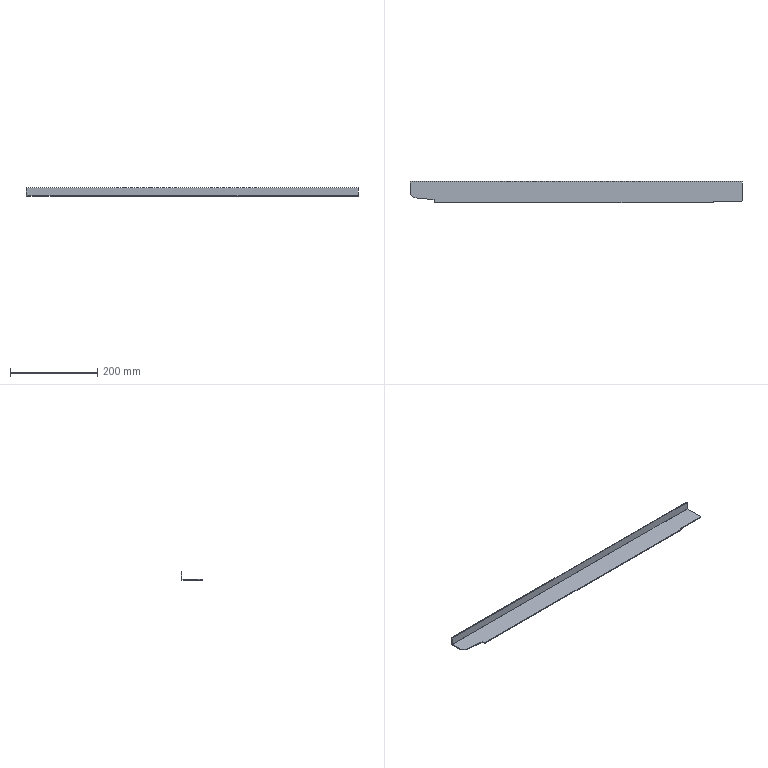Part | SolidWorks | 1 solid | 21 faces | box 759.5 x 50 x 20 mm | volume 100833 mm3 | plane 19 | cylinder 2 | commonest cylinder face diameters 0.2 x1 4.2 x1
STEP:
#1=CARTESIAN_POINT('',(-379.75,22.9,-2.));
#2=VERTEX_POINT('',#1);
#3=CARTESIAN_POINT('',(-379.75,-3.027,-2.));
#4=VERTEX_POINT('',#3);
#5=CARTESIAN_POINT('',(-379.75,-25.,-2.));
#6=DIRECTION('',(0.,-1.,0.));
#7=VECTOR('',#6,1000.);
#8=LINE('',#5,#7);
#9=EDGE_CURVE('',#2,#4,#8,.T.);
#10=ORIENTED_EDGE('',*,*,#9,.T.);
#11=CARTESIAN_POINT('',(-379.75,-3.027,0.));
#12=VERTEX_POINT('',#11);
#13=CARTESIAN_POINT('',(-379.75,-3.027,-2.));
#14=DIRECTION('',(0.,0.,1.));
#15=VECTOR('',#14,1000.);
#16=LINE('',#13,#15);
#17=EDGE_CURVE('',#4,#12,#16,.T.);
#18=ORIENTED_EDGE('',*,*,#17,.T.);
#19=CARTESIAN_POINT('',(-379.75,22.9,0.));
#20=VERTEX_POINT('',#19);
#21=CARTESIAN_POINT('',(-379.75,-25.,0.));
#22=DIRECTION('',(0.,-1.,0.));
#23=VECTOR('',#22,1000.);
#24=LINE('',#21,#23);
#25=EDGE_CURVE('',#20,#12,#24,.T.);
#26=ORIENTED_EDGE('',*,*,#25,.F.);
#27=CARTESIAN_POINT('',(-379.75,22.9,0.));
#28=DIRECTION('',(0.,0.,-1.));
#29=VECTOR('',#28,1000.);
#30=LINE('',#27,#29);
#31=EDGE_CURVE('',#20,#2,#30,.T.);
#32=ORIENTED_EDGE('',*,*,#31,.T.);
#33=EDGE_LOOP('',(#10,#18,#26,#32));
#34=FACE_OUTER_BOUND('',#33,.T.);
#35=CARTESIAN_POINT('',(-379.75,-25.,-2.));
#36=DIRECTION('',(-1.,0.,0.));
#37=DIRECTION('',(0.,0.,1.));
#38=AXIS2_PLACEMENT_3D('',#35,#36,#37);
#39=PLANE('',#38);
#40=ADVANCED_FACE('',(#34),#39,.T.);
#41=CARTESIAN_POINT('',(-323.25,-25.,-2.));
#42=VERTEX_POINT('',#41);
#43=CARTESIAN_POINT('',(-323.25,-17.499,-2.));
#44=VERTEX_POINT('',#43);
#45=CARTESIAN_POINT('',(-323.25,0.,-2.));
#46=DIRECTION('',(0.,1.,0.));
#47=VECTOR('',#46,1000.);
#48=LINE('',#45,#47);
#49=EDGE_CURVE('',#42,#44,#48,.T.);
#50=ORIENTED_EDGE('',*,*,#49,.T.);
#51=CARTESIAN_POINT('',(-327.727,-17.499,-2.));
#52=VERTEX_POINT('',#51);
#53=CARTESIAN_POINT('',(0.,-17.499,-2.));
#54=DIRECTION('',(-1.,0.,0.));
#55=VECTOR('',#54,1000.);
#56=LINE('',#53,#55);
#57=EDGE_CURVE('',#44,#52,#56,.T.);
#58=ORIENTED_EDGE('',*,*,#57,.T.);
#59=CARTESIAN_POINT('',(-370.795,-12.972,-2.));
#60=VERTEX_POINT('',#59);
#61=CARTESIAN_POINT('',(-5.4,-51.377,-2.));
#62=DIRECTION('',(-0.9945,0.1045,0.));
#63=VECTOR('',#62,1000.);
#64=LINE('',#61,#63);
#65=EDGE_CURVE('',#52,#60,#64,.T.);
#66=ORIENTED_EDGE('',*,*,#65,.T.);
#67=CARTESIAN_POINT('',(-211.227,-190.19,-2.));
#68=DIRECTION('',(-0.6691,0.7431,0.));
#69=VECTOR('',#68,1000.);
#70=LINE('',#67,#69);
#71=EDGE_CURVE('',#60,#4,#70,.T.);
#72=ORIENTED_EDGE('',*,*,#71,.T.);
#73=ORIENTED_EDGE('',*,*,#9,.F.);
#74=CARTESIAN_POINT('',(379.75,22.9,-2.));
#75=VERTEX_POINT('',#74);
#76=CARTESIAN_POINT('',(-379.75,22.9,-2.));
#77=DIRECTION('',(1.,0.,0.));
#78=VECTOR('',#77,1000.);
#79=LINE('',#76,#78);
#80=EDGE_CURVE('',#2,#75,#79,.T.);
#81=ORIENTED_EDGE('',*,*,#80,.T.);
#82=CARTESIAN_POINT('',(379.75,-20.,-2.));
#83=VERTEX_POINT('',#82);
#84=CARTESIAN_POINT('',(379.75,-25.,-2.));
#85=DIRECTION('',(0.,1.,0.));
#86=VECTOR('',#85,1000.);
#87=LINE('',#84,#86);
#88=EDGE_CURVE('',#83,#75,#87,.T.);
#89=ORIENTED_EDGE('',*,*,#88,.F.);
#90=CARTESIAN_POINT('',(378.75,-21.,-2.));
#91=VERTEX_POINT('',#90);
#92=CARTESIAN_POINT('',(199.875,-199.875,-2.));
#93=DIRECTION('',(-0.7071,-0.7071,0.));
#94=VECTOR('',#93,1000.);
#95=LINE('',#92,#94);
#96=EDGE_CURVE('',#83,#91,#95,.T.);
#97=ORIENTED_EDGE('',*,*,#96,.T.);
#98=CARTESIAN_POINT('',(313.75,-21.,-2.));
#99=VERTEX_POINT('',#98);
#100=CARTESIAN_POINT('',(0.,-21.,-2.));
#101=DIRECTION('',(-1.,0.,0.));
#102=VECTOR('',#101,1000.);
#103=LINE('',#100,#102);
#104=EDGE_CURVE('',#91,#99,#103,.T.);
#105=ORIENTED_EDGE('',*,*,#104,.T.);
#106=CARTESIAN_POINT('',(313.75,-25.,-2.));
#107=VERTEX_POINT('',#106);
#108=CARTESIAN_POINT('',(313.75,0.,-2.));
#109=DIRECTION('',(0.,-1.,0.));
#110=VECTOR('',#109,1000.);
#111=LINE('',#108,#110);
#112=EDGE_CURVE('',#99,#107,#111,.T.);
#113=ORIENTED_EDGE('',*,*,#112,.T.);
#114=CARTESIAN_POINT('',(379.75,-25.,-2.));
#115=DIRECTION('',(1.,0.,0.));
#116=VECTOR('',#115,1000.);
#117=LINE('',#114,#116);
#118=EDGE_CURVE('',#42,#107,#117,.T.);
#119=ORIENTED_EDGE('',*,*,#118,.F.);
#120=EDGE_LOOP('',(#50,#58,#66,#72,#73,#81,#89,#97,#105,#113,#119));
#121=FACE_OUTER_BOUND('',#120,.T.);
#122=CARTESIAN_POINT('',(0.,0.,-2.));
#123=DIRECTION('',(0.,0.,1.));
#124=DIRECTION('',(1.,0.,0.));
#125=AXIS2_PLACEMENT_3D('',#122,#123,#124);
#126=PLANE('',#125);
#127=ADVANCED_FACE('',(#121),#126,.F.);
#128=CARTESIAN_POINT('',(-323.25,-17.499,0.));
#129=VERTEX_POINT('',#128);
#130=CARTESIAN_POINT('',(-327.727,-17.499,0.));
#131=VERTEX_POINT('',#130);
#132=CARTESIAN_POINT('',(0.,-17.499,0.));
#133=DIRECTION('',(-1.,0.,0.));
#134=VECTOR('',#133,1000.);
#135=LINE('',#132,#134);
#136=EDGE_CURVE('',#129,#131,#135,.T.);
#137=ORIENTED_EDGE('',*,*,#136,.F.);
#138=CARTESIAN_POINT('',(-323.25,-25.,0.));
#139=VERTEX_POINT('',#138);
#140=CARTESIAN_POINT('',(-323.25,0.,0.));
#141=DIRECTION('',(0.,1.,0.));
#142=VECTOR('',#141,1000.);
#143=LINE('',#140,#142);
#144=EDGE_CURVE('',#139,#129,#143,.T.);
#145=ORIENTED_EDGE('',*,*,#144,.F.);
#146=CARTESIAN_POINT('',(313.75,-25.,0.));
#147=VERTEX_POINT('',#146);
#148=CARTESIAN_POINT('',(379.75,-25.,0.));
#149=DIRECTION('',(1.,0.,0.));
#150=VECTOR('',#149,1000.);
#151=LINE('',#148,#150);
#152=EDGE_CURVE('',#139,#147,#151,.T.);
#153=ORIENTED_EDGE('',*,*,#152,.T.);
#154=CARTESIAN_POINT('',(313.75,-21.,0.));
#155=VERTEX_POINT('',#154);
#156=CARTESIAN_POINT('',(313.75,0.,0.));
#157=DIRECTION('',(0.,-1.,0.));
#158=VECTOR('',#157,1000.);
#159=LINE('',#156,#158);
#160=EDGE_CURVE('',#155,#147,#159,.T.);
#161=ORIENTED_EDGE('',*,*,#160,.F.);
#162=CARTESIAN_POINT('',(378.75,-21.,0.));
#163=VERTEX_POINT('',#162);
#164=CARTESIAN_POINT('',(0.,-21.,0.));
#165=DIRECTION('',(-1.,0.,0.));
#166=VECTOR('',#165,1000.);
#167=LINE('',#164,#166);
#168=EDGE_CURVE('',#163,#155,#167,.T.);
#169=ORIENTED_EDGE('',*,*,#168,.F.);
#170=CARTESIAN_POINT('',(379.75,-20.,0.));
#171=VERTEX_POINT('',#170);
#172=CARTESIAN_POINT('',(199.875,-199.875,0.));
#173=DIRECTION('',(-0.7071,-0.7071,0.));
#174=VECTOR('',#173,1000.);
#175=LINE('',#172,#174);
#176=EDGE_CURVE('',#171,#163,#175,.T.);
#177=ORIENTED_EDGE('',*,*,#176,.F.);
#178=CARTESIAN_POINT('',(379.75,22.9,0.));
#179=VERTEX_POINT('',#178);
#180=CARTESIAN_POINT('',(379.75,-25.,0.));
#181=DIRECTION('',(0.,1.,0.));
#182=VECTOR('',#181,1000.);
#183=LINE('',#180,#182);
#184=EDGE_CURVE('',#171,#179,#183,.T.);
#185=ORIENTED_EDGE('',*,*,#184,.T.);
#186=CARTESIAN_POINT('',(-379.75,22.9,0.));
#187=DIRECTION('',(1.,0.,0.));
#188=VECTOR('',#187,1000.);
#189=LINE('',#186,#188);
#190=EDGE_CURVE('',#20,#179,#189,.T.);
#191=ORIENTED_EDGE('',*,*,#190,.F.);
#192=ORIENTED_EDGE('',*,*,#25,.T.);
#193=CARTESIAN_POINT('',(-370.795,-12.972,0.));
#194=VERTEX_POINT('',#193);
#195=CARTESIAN_POINT('',(-211.227,-190.19,0.));
#196=DIRECTION('',(-0.6691,0.7431,0.));
#197=VECTOR('',#196,1000.);
#198=LINE('',#195,#197);
#199=EDGE_CURVE('',#194,#12,#198,.T.);
#200=ORIENTED_EDGE('',*,*,#199,.F.);
#201=CARTESIAN_POINT('',(-5.4,-51.377,0.));
#202=DIRECTION('',(-0.9945,0.1045,0.));
#203=VECTOR('',#202,1000.);
#204=LINE('',#201,#203);
#205=EDGE_CURVE('',#131,#194,#204,.T.);
#206=ORIENTED_EDGE('',*,*,#205,.F.);
#207=EDGE_LOOP('',(#137,#145,#153,#161,#169,#177,#185,#191,#192,#200,#206));
#208=FACE_OUTER_BOUND('',#207,.T.);
#209=CARTESIAN_POINT('',(0.,0.,0.));
#210=DIRECTION('',(0.,0.,1.));
#211=DIRECTION('',(1.,0.,0.));
#212=AXIS2_PLACEMENT_3D('',#209,#210,#211);
#213=PLANE('',#212);
#214=ADVANCED_FACE('',(#208),#213,.T.);
#215=ORIENTED_EDGE('',*,*,#184,.F.);
#216=CARTESIAN_POINT('',(379.75,-20.,-2.));
#217=DIRECTION('',(0.,0.,1.));
#218=VECTOR('',#217,1000.);
#219=LINE('',#216,#218);
#220=EDGE_CURVE('',#83,#171,#219,.T.);
#221=ORIENTED_EDGE('',*,*,#220,.F.);
#222=ORIENTED_EDGE('',*,*,#88,.T.);
#223=CARTESIAN_POINT('',(379.75,22.9,0.));
#224=DIRECTION('',(0.,0.,-1.));
#225=VECTOR('',#224,1000.);
#226=LINE('',#223,#225);
#227=EDGE_CURVE('',#179,#75,#226,.T.);
#228=ORIENTED_EDGE('',*,*,#227,.F.);
#229=EDGE_LOOP('',(#215,#221,#222,#228));
#230=FACE_OUTER_BOUND('',#229,.T.);
#231=CARTESIAN_POINT('',(379.75,-25.,-2.));
#232=DIRECTION('',(1.,0.,0.));
#233=DIRECTION('',(0.,0.,-1.));
#234=AXIS2_PLACEMENT_3D('',#231,#232,#233);
#235=PLANE('',#234);
#236=ADVANCED_FACE('',(#230),#235,.T.);
#237=ORIENTED_EDGE('',*,*,#152,.F.);
#238=CARTESIAN_POINT('',(-323.25,-25.,-2.));
#239=DIRECTION('',(0.,0.,1.));
#240=VECTOR('',#239,1000.);
#241=LINE('',#238,#240);
#242=EDGE_CURVE('',#42,#139,#241,.T.);
#243=ORIENTED_EDGE('',*,*,#242,.F.);
#244=ORIENTED_EDGE('',*,*,#118,.T.);
#245=CARTESIAN_POINT('',(313.75,-25.,-2.));
#246=DIRECTION('',(0.,0.,1.));
#247=VECTOR('',#246,1000.);
#248=LINE('',#245,#247);
#249=EDGE_CURVE('',#107,#147,#248,.T.);
#250=ORIENTED_EDGE('',*,*,#249,.T.);
#251=EDGE_LOOP('',(#237,#243,#244,#250));
#252=FACE_OUTER_BOUND('',#251,.T.);
#253=CARTESIAN_POINT('',(379.75,-25.,-2.));
#254=DIRECTION('',(0.,-1.,0.));
#255=DIRECTION('',(1.,0.,0.));
#256=AXIS2_PLACEMENT_3D('',#253,#254,#255);
#257=PLANE('',#256);
#258=ADVANCED_FACE('',(#252),#257,.T.);
#259=CARTESIAN_POINT('',(379.75,23.,0.1));
#260=VERTEX_POINT('',#259);
#261=CARTESIAN_POINT('',(379.75,25.,0.1));
#262=VERTEX_POINT('',#261);
#263=CARTESIAN_POINT('',(379.75,25.,0.1));
#264=DIRECTION('',(0.,1.,0.));
#265=VECTOR('',#264,1000.);
#266=LINE('',#263,#265);
#267=EDGE_CURVE('',#260,#262,#266,.T.);
#268=ORIENTED_EDGE('',*,*,#267,.F.);
#269=CARTESIAN_POINT('',(379.75,22.9,0.1));
#270=DIRECTION('',(1.,0.,0.));
#271=DIRECTION('',(0.,0.,1.));
#272=AXIS2_PLACEMENT_3D('',#269,#270,#271);
#273=CIRCLE('',#272,0.1);
#274=EDGE_CURVE('',#179,#260,#273,.T.);
#275=ORIENTED_EDGE('',*,*,#274,.F.);
#276=ORIENTED_EDGE('',*,*,#227,.T.);
#277=CARTESIAN_POINT('',(379.75,22.9,0.1));
#278=DIRECTION('',(1.,0.,0.));
#279=DIRECTION('',(0.,0.,1.));
#280=AXIS2_PLACEMENT_3D('',#277,#278,#279);
#281=CIRCLE('',#280,2.1);
#282=EDGE_CURVE('',#75,#262,#281,.T.);
#283=ORIENTED_EDGE('',*,*,#282,.T.);
#284=EDGE_LOOP('',(#268,#275,#276,#283));
#285=FACE_OUTER_BOUND('',#284,.T.);
#286=CARTESIAN_POINT('',(379.75,22.9,0.1));
#287=DIRECTION('',(1.,0.,0.));
#288=DIRECTION('',(0.,0.,-1.));
#289=AXIS2_PLACEMENT_3D('',#286,#287,#288);
#290=PLANE('',#289);
#291=ADVANCED_FACE('',(#285),#290,.T.);
#292=CARTESIAN_POINT('',(-379.75,23.,0.1));
#293=VERTEX_POINT('',#292);
#294=CARTESIAN_POINT('',(-379.75,22.9,0.1));
#295=DIRECTION('',(-1.,0.,0.));
#296=DIRECTION('',(0.,0.,1.));
#297=AXIS2_PLACEMENT_3D('',#294,#295,#296);
#298=CIRCLE('',#297,0.1);
#299=EDGE_CURVE('',#293,#20,#298,.T.);
#300=ORIENTED_EDGE('',*,*,#299,.F.);
#301=CARTESIAN_POINT('',(-379.75,25.,0.1));
#302=VERTEX_POINT('',#301);
#303=CARTESIAN_POINT('',(-379.75,23.,0.1));
#304=DIRECTION('',(0.,1.,0.));
#305=VECTOR('',#304,1000.);
#306=LINE('',#303,#305);
#307=EDGE_CURVE('',#293,#302,#306,.T.);
#308=ORIENTED_EDGE('',*,*,#307,.T.);
#309=CARTESIAN_POINT('',(-379.75,22.9,0.1));
#310=DIRECTION('',(-1.,0.,0.));
#311=DIRECTION('',(0.,0.,1.));
#312=AXIS2_PLACEMENT_3D('',#309,#310,#311);
#313=CIRCLE('',#312,2.1);
#314=EDGE_CURVE('',#302,#2,#313,.T.);
#315=ORIENTED_EDGE('',*,*,#314,.T.);
#316=ORIENTED_EDGE('',*,*,#31,.F.);
#317=EDGE_LOOP('',(#300,#308,#315,#316));
#318=FACE_OUTER_BOUND('',#317,.T.);
#319=CARTESIAN_POINT('',(-379.75,22.9,0.1));
#320=DIRECTION('',(1.,0.,0.));
#321=DIRECTION('',(0.,0.,-1.));
#322=AXIS2_PLACEMENT_3D('',#319,#320,#321);
#323=PLANE('',#322);
#324=ADVANCED_FACE('',(#318),#323,.F.);
#325=ORIENTED_EDGE('',*,*,#80,.F.);
#326=ORIENTED_EDGE('',*,*,#314,.F.);
#327=CARTESIAN_POINT('',(379.75,25.,0.1));
#328=DIRECTION('',(1.,0.,0.));
#329=VECTOR('',#328,1000.);
#330=LINE('',#327,#329);
#331=EDGE_CURVE('',#302,#262,#330,.T.);
#332=ORIENTED_EDGE('',*,*,#331,.T.);
#333=ORIENTED_EDGE('',*,*,#282,.F.);
#334=EDGE_LOOP('',(#325,#326,#332,#333));
#335=FACE_OUTER_BOUND('',#334,.T.);
#336=CARTESIAN_POINT('',(-379.75,22.9,0.1));
#337=DIRECTION('',(-1.,0.,0.));
#338=DIRECTION('',(0.,1.,0.));
#339=AXIS2_PLACEMENT_3D('',#336,#337,#338);
#340=CYLINDRICAL_SURFACE('',#339,2.1);
#341=ADVANCED_FACE('',(#335),#340,.T.);
#342=ORIENTED_EDGE('',*,*,#190,.T.);
#343=ORIENTED_EDGE('',*,*,#274,.T.);
#344=CARTESIAN_POINT('',(379.75,23.,0.1));
#345=DIRECTION('',(-1.,0.,0.));
#346=VECTOR('',#345,1000.);
#347=LINE('',#344,#346);
#348=EDGE_CURVE('',#260,#293,#347,.T.);
#349=ORIENTED_EDGE('',*,*,#348,.T.);
#350=ORIENTED_EDGE('',*,*,#299,.T.);
#351=EDGE_LOOP('',(#342,#343,#349,#350));
#352=FACE_OUTER_BOUND('',#351,.T.);
#353=CARTESIAN_POINT('',(-379.75,22.9,0.1));
#354=DIRECTION('',(-1.,0.,0.));
#355=DIRECTION('',(0.,1.,0.));
#356=AXIS2_PLACEMENT_3D('',#353,#354,#355);
#357=CYLINDRICAL_SURFACE('',#356,0.1);
#358=ADVANCED_FACE('',(#352),#357,.F.);
#359=ORIENTED_EDGE('',*,*,#267,.T.);
#360=CARTESIAN_POINT('',(379.75,25.,18.));
#361=VERTEX_POINT('',#360);
#362=CARTESIAN_POINT('',(379.75,25.,0.));
#363=DIRECTION('',(0.,0.,-1.));
#364=VECTOR('',#363,1000.);
#365=LINE('',#362,#364);
#366=EDGE_CURVE('',#361,#262,#365,.T.);
#367=ORIENTED_EDGE('',*,*,#366,.F.);
#368=CARTESIAN_POINT('',(379.75,23.,18.));
#369=VERTEX_POINT('',#368);
#370=CARTESIAN_POINT('',(379.75,25.,18.));
#371=DIRECTION('',(0.,-1.,0.));
#372=VECTOR('',#371,1000.);
#373=LINE('',#370,#372);
#374=EDGE_CURVE('',#361,#369,#373,.T.);
#375=ORIENTED_EDGE('',*,*,#374,.T.);
#376=CARTESIAN_POINT('',(379.75,23.,0.));
#377=DIRECTION('',(0.,0.,-1.));
#378=VECTOR('',#377,1000.);
#379=LINE('',#376,#378);
#380=EDGE_CURVE('',#369,#260,#379,.T.);
#381=ORIENTED_EDGE('',*,*,#380,.T.);
#382=EDGE_LOOP('',(#359,#367,#375,#381));
#383=FACE_OUTER_BOUND('',#382,.T.);
#384=CARTESIAN_POINT('',(379.75,25.,0.));
#385=DIRECTION('',(-1.,0.,0.));
#386=DIRECTION('',(0.,-1.,0.));
#387=AXIS2_PLACEMENT_3D('',#384,#385,#386);
#388=PLANE('',#387);
#389=ADVANCED_FACE('',(#383),#388,.F.);
#390=ORIENTED_EDGE('',*,*,#307,.F.);
#391=CARTESIAN_POINT('',(-379.75,23.,18.));
#392=VERTEX_POINT('',#391);
#393=CARTESIAN_POINT('',(-379.75,23.,18.));
#394=DIRECTION('',(0.,0.,1.));
#395=VECTOR('',#394,1000.);
#396=LINE('',#393,#395);
#397=EDGE_CURVE('',#293,#392,#396,.T.);
#398=ORIENTED_EDGE('',*,*,#397,.T.);
#399=CARTESIAN_POINT('',(-379.75,25.,18.));
#400=VERTEX_POINT('',#399);
#401=CARTESIAN_POINT('',(-379.75,25.,18.));
#402=DIRECTION('',(0.,-1.,0.));
#403=VECTOR('',#402,1000.);
#404=LINE('',#401,#403);
#405=EDGE_CURVE('',#400,#392,#404,.T.);
#406=ORIENTED_EDGE('',*,*,#405,.F.);
#407=CARTESIAN_POINT('',(-379.75,25.,0.));
#408=DIRECTION('',(0.,0.,1.));
#409=VECTOR('',#408,1000.);
#410=LINE('',#407,#409);
#411=EDGE_CURVE('',#302,#400,#410,.T.);
#412=ORIENTED_EDGE('',*,*,#411,.F.);
#413=EDGE_LOOP('',(#390,#398,#406,#412));
#414=FACE_OUTER_BOUND('',#413,.T.);
#415=CARTESIAN_POINT('',(-379.75,25.,18.));
#416=DIRECTION('',(1.,0.,0.));
#417=DIRECTION('',(0.,1.,0.));
#418=AXIS2_PLACEMENT_3D('',#415,#416,#417);
#419=PLANE('',#418);
#420=ADVANCED_FACE('',(#414),#419,.F.);
#421=ORIENTED_EDGE('',*,*,#331,.F.);
#422=ORIENTED_EDGE('',*,*,#411,.T.);
#423=CARTESIAN_POINT('',(0.,25.,18.));
#424=DIRECTION('',(1.,0.,0.));
#425=VECTOR('',#424,1000.);
#426=LINE('',#423,#425);
#427=EDGE_CURVE('',#400,#361,#426,.T.);
#428=ORIENTED_EDGE('',*,*,#427,.T.);
#429=ORIENTED_EDGE('',*,*,#366,.T.);
#430=EDGE_LOOP('',(#421,#422,#428,#429));
#431=FACE_OUTER_BOUND('',#430,.T.);
#432=CARTESIAN_POINT('',(0.,25.,0.));
#433=DIRECTION('',(0.,-1.,0.));
#434=DIRECTION('',(0.,0.,-1.));
#435=AXIS2_PLACEMENT_3D('',#432,#433,#434);
#436=PLANE('',#435);
#437=ADVANCED_FACE('',(#431),#436,.F.);
#438=ORIENTED_EDGE('',*,*,#397,.F.);
#439=ORIENTED_EDGE('',*,*,#348,.F.);
#440=ORIENTED_EDGE('',*,*,#380,.F.);
#441=CARTESIAN_POINT('',(379.75,23.,18.));
#442=DIRECTION('',(1.,0.,0.));
#443=VECTOR('',#442,1000.);
#444=LINE('',#441,#443);
#445=EDGE_CURVE('',#392,#369,#444,.T.);
#446=ORIENTED_EDGE('',*,*,#445,.F.);
#447=EDGE_LOOP('',(#438,#439,#440,#446));
#448=FACE_OUTER_BOUND('',#447,.T.);
#449=CARTESIAN_POINT('',(0.,23.,0.));
#450=DIRECTION('',(0.,-1.,0.));
#451=DIRECTION('',(0.,0.,-1.));
#452=AXIS2_PLACEMENT_3D('',#449,#450,#451);
#453=PLANE('',#452);
#454=ADVANCED_FACE('',(#448),#453,.T.);
#455=ORIENTED_EDGE('',*,*,#445,.T.);
#456=ORIENTED_EDGE('',*,*,#374,.F.);
#457=ORIENTED_EDGE('',*,*,#427,.F.);
#458=ORIENTED_EDGE('',*,*,#405,.T.);
#459=EDGE_LOOP('',(#455,#456,#457,#458));
#460=FACE_OUTER_BOUND('',#459,.T.);
#461=CARTESIAN_POINT('',(379.75,25.,18.));
#462=DIRECTION('',(0.,0.,-1.));
#463=DIRECTION('',(0.,1.,0.));
#464=AXIS2_PLACEMENT_3D('',#461,#462,#463);
#465=PLANE('',#464);
#466=ADVANCED_FACE('',(#460),#465,.F.);
#467=ORIENTED_EDGE('',*,*,#249,.F.);
#468=ORIENTED_EDGE('',*,*,#112,.F.);
#469=CARTESIAN_POINT('',(313.75,-21.,-2.));
#470=DIRECTION('',(0.,0.,1.));
#471=VECTOR('',#470,1000.);
#472=LINE('',#469,#471);
#473=EDGE_CURVE('',#99,#155,#472,.T.);
#474=ORIENTED_EDGE('',*,*,#473,.T.);
#475=ORIENTED_EDGE('',*,*,#160,.T.);
#476=EDGE_LOOP('',(#467,#468,#474,#475));
#477=FACE_OUTER_BOUND('',#476,.T.);
#478=CARTESIAN_POINT('',(313.75,0.,-2.));
#479=DIRECTION('',(-1.,0.,0.));
#480=DIRECTION('',(0.,-1.,0.));
#481=AXIS2_PLACEMENT_3D('',#478,#479,#480);
#482=PLANE('',#481);
#483=ADVANCED_FACE('',(#477),#482,.F.);
#484=ORIENTED_EDGE('',*,*,#473,.F.);
#485=ORIENTED_EDGE('',*,*,#104,.F.);
#486=CARTESIAN_POINT('',(378.75,-21.,-2.));
#487=DIRECTION('',(0.,0.,1.));
#488=VECTOR('',#487,1000.);
#489=LINE('',#486,#488);
#490=EDGE_CURVE('',#91,#163,#489,.T.);
#491=ORIENTED_EDGE('',*,*,#490,.T.);
#492=ORIENTED_EDGE('',*,*,#168,.T.);
#493=EDGE_LOOP('',(#484,#485,#491,#492));
#494=FACE_OUTER_BOUND('',#493,.T.);
#495=CARTESIAN_POINT('',(0.,-21.,-2.));
#496=DIRECTION('',(0.,1.,0.));
#497=DIRECTION('',(-1.,0.,0.));
#498=AXIS2_PLACEMENT_3D('',#495,#496,#497);
#499=PLANE('',#498);
#500=ADVANCED_FACE('',(#494),#499,.F.);
#501=ORIENTED_EDGE('',*,*,#490,.F.);
#502=ORIENTED_EDGE('',*,*,#96,.F.);
#503=ORIENTED_EDGE('',*,*,#220,.T.);
#504=ORIENTED_EDGE('',*,*,#176,.T.);
#505=EDGE_LOOP('',(#501,#502,#503,#504));
#506=FACE_OUTER_BOUND('',#505,.T.);
#507=CARTESIAN_POINT('',(199.875,-199.875,-2.));
#508=DIRECTION('',(-0.7071,0.7071,0.));
#509=DIRECTION('',(-0.7071,-0.7071,0.));
#510=AXIS2_PLACEMENT_3D('',#507,#508,#509);
#511=PLANE('',#510);
#512=ADVANCED_FACE('',(#506),#511,.F.);
#513=CARTESIAN_POINT('',(-327.727,-17.499,-2.));
#514=DIRECTION('',(0.,0.,1.));
#515=VECTOR('',#514,1000.);
#516=LINE('',#513,#515);
#517=EDGE_CURVE('',#52,#131,#516,.T.);
#518=ORIENTED_EDGE('',*,*,#517,.F.);
#519=ORIENTED_EDGE('',*,*,#57,.F.);
#520=CARTESIAN_POINT('',(-323.25,-17.499,-2.));
#521=DIRECTION('',(0.,0.,1.));
#522=VECTOR('',#521,1000.);
#523=LINE('',#520,#522);
#524=EDGE_CURVE('',#44,#129,#523,.T.);
#525=ORIENTED_EDGE('',*,*,#524,.T.);
#526=ORIENTED_EDGE('',*,*,#136,.T.);
#527=EDGE_LOOP('',(#518,#519,#525,#526));
#528=FACE_OUTER_BOUND('',#527,.T.);
#529=CARTESIAN_POINT('',(0.,-17.499,-2.));
#530=DIRECTION('',(0.,1.,0.));
#531=DIRECTION('',(-1.,0.,0.));
#532=AXIS2_PLACEMENT_3D('',#529,#530,#531);
#533=PLANE('',#532);
#534=ADVANCED_FACE('',(#528),#533,.F.);
#535=ORIENTED_EDGE('',*,*,#524,.F.);
#536=ORIENTED_EDGE('',*,*,#49,.F.);
#537=ORIENTED_EDGE('',*,*,#242,.T.);
#538=ORIENTED_EDGE('',*,*,#144,.T.);
#539=EDGE_LOOP('',(#535,#536,#537,#538));
#540=FACE_OUTER_BOUND('',#539,.T.);
#541=CARTESIAN_POINT('',(-323.25,0.,-2.));
#542=DIRECTION('',(1.,0.,0.));
#543=DIRECTION('',(0.,1.,0.));
#544=AXIS2_PLACEMENT_3D('',#541,#542,#543);
#545=PLANE('',#544);
#546=ADVANCED_FACE('',(#540),#545,.F.);
#547=ORIENTED_EDGE('',*,*,#17,.F.);
#548=ORIENTED_EDGE('',*,*,#71,.F.);
#549=CARTESIAN_POINT('',(-370.795,-12.972,-2.));
#550=DIRECTION('',(0.,0.,1.));
#551=VECTOR('',#550,1000.);
#552=LINE('',#549,#551);
#553=EDGE_CURVE('',#60,#194,#552,.T.);
#554=ORIENTED_EDGE('',*,*,#553,.T.);
#555=ORIENTED_EDGE('',*,*,#199,.T.);
#556=EDGE_LOOP('',(#547,#548,#554,#555));
#557=FACE_OUTER_BOUND('',#556,.T.);
#558=CARTESIAN_POINT('',(-211.227,-190.19,-2.));
#559=DIRECTION('',(0.7431,0.6691,0.));
#560=DIRECTION('',(-0.6691,0.7431,0.));
#561=AXIS2_PLACEMENT_3D('',#558,#559,#560);
#562=PLANE('',#561);
#563=ADVANCED_FACE('',(#557),#562,.F.);
#564=ORIENTED_EDGE('',*,*,#65,.F.);
#565=ORIENTED_EDGE('',*,*,#517,.T.);
#566=ORIENTED_EDGE('',*,*,#205,.T.);
#567=ORIENTED_EDGE('',*,*,#553,.F.);
#568=EDGE_LOOP('',(#564,#565,#566,#567));
#569=FACE_OUTER_BOUND('',#568,.T.);
#570=CARTESIAN_POINT('',(-5.4,-51.377,-2.));
#571=DIRECTION('',(0.1045,0.9945,0.));
#572=DIRECTION('',(-0.9945,0.1045,0.));
#573=AXIS2_PLACEMENT_3D('',#570,#571,#572);
#574=PLANE('',#573);
#575=ADVANCED_FACE('',(#569),#574,.F.);
#576=CLOSED_SHELL('',(#40,#127,#214,#236,#258,#291,#324,#341,#358,#389,#420,#437,#454,#466,#483,#500,#512,#534,#546,#563,#575));
#577=MANIFOLD_SOLID_BREP('',#576);
#578=CARTESIAN_POINT('',(0.,0.,0.));
#579=DIRECTION('',(0.,0.,1.));
#580=DIRECTION('',(1.,0.,0.));
#581=AXIS2_PLACEMENT_3D('',#578,#579,#580);
#582=(LENGTH_UNIT()NAMED_UNIT(*)SI_UNIT(.MILLI.,.METRE.));
#583=UNCERTAINTY_MEASURE_WITH_UNIT(LENGTH_MEASURE(0.00001),#582,'','');
#584=(NAMED_UNIT(*)PLANE_ANGLE_UNIT()SI_UNIT($,.RADIAN.));
#585=(NAMED_UNIT(*)SI_UNIT($,.STERADIAN.)SOLID_ANGLE_UNIT());
#586=(GEOMETRIC_REPRESENTATION_CONTEXT(3)GLOBAL_UNCERTAINTY_ASSIGNED_CONTEXT((#583))GLOBAL_UNIT_ASSIGNED_CONTEXT((#582,#584,#585))REPRESENTATION_CONTEXT('',''));
#587=ADVANCED_BREP_SHAPE_REPRESENTATION('',(#577,#581),#586);